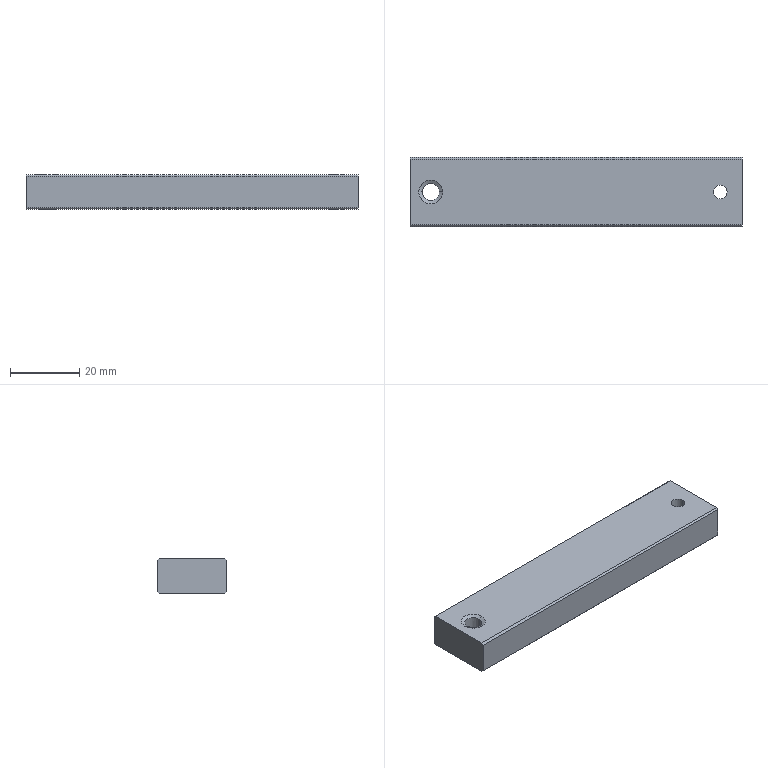Part | NX | 1 solid | 30 faces | box 96 x 20 x 10 mm | volume 18717 mm3 | cylinder 12 | plane 10 | cone 8 | commonest cylinder face diameters 3.3 x8 4 x2 5 x2
STEP:
#1=CARTESIAN_POINT('',(-48.,-9.5,5.));
#2=VERTEX_POINT('',#1);
#3=CARTESIAN_POINT('',(48.,-9.5,5.));
#4=VERTEX_POINT('',#3);
#5=CARTESIAN_POINT('',(0.,-9.5,5.));
#6=DIRECTION('',(1.,0.,0.));
#7=VECTOR('',#6,1000.);
#8=LINE('',#5,#7);
#9=EDGE_CURVE('',#2,#4,#8,.T.);
#10=ORIENTED_EDGE('',*,*,#9,.T.);
#11=CARTESIAN_POINT('',(48.,9.5,5.));
#12=VERTEX_POINT('',#11);
#13=CARTESIAN_POINT('',(48.,0.,5.));
#14=DIRECTION('',(0.,-1.,0.));
#15=VECTOR('',#14,1000.);
#16=LINE('',#13,#15);
#17=EDGE_CURVE('',#12,#4,#16,.T.);
#18=ORIENTED_EDGE('',*,*,#17,.F.);
#19=CARTESIAN_POINT('',(-48.,9.5,5.));
#20=VERTEX_POINT('',#19);
#21=CARTESIAN_POINT('',(0.,9.5,5.));
#22=DIRECTION('',(-1.,0.,0.));
#23=VECTOR('',#22,1000.);
#24=LINE('',#21,#23);
#25=EDGE_CURVE('',#12,#20,#24,.T.);
#26=ORIENTED_EDGE('',*,*,#25,.T.);
#27=CARTESIAN_POINT('',(-48.,0.,5.));
#28=DIRECTION('',(0.,1.,0.));
#29=VECTOR('',#28,1000.);
#30=LINE('',#27,#29);
#31=EDGE_CURVE('',#2,#20,#30,.T.);
#32=ORIENTED_EDGE('',*,*,#31,.F.);
#33=EDGE_LOOP('',(#10,#18,#26,#32));
#34=FACE_BOUND('',#33,.T.);
#35=CARTESIAN_POINT('',(43.7,0.,5.));
#36=VERTEX_POINT('',#35);
#37=CARTESIAN_POINT('',(39.7,0.,5.));
#38=VERTEX_POINT('',#37);
#39=CARTESIAN_POINT('',(41.7,0.,5.));
#40=DIRECTION('',(0.,0.,-1.));
#41=DIRECTION('',(-1.,0.,0.));
#42=AXIS2_PLACEMENT_3D('',#39,#40,#41);
#43=CIRCLE('',#42,2.);
#44=EDGE_CURVE('',#36,#38,#43,.T.);
#45=ORIENTED_EDGE('',*,*,#44,.T.);
#46=CARTESIAN_POINT('',(41.7,0.,5.));
#47=DIRECTION('',(0.,0.,-1.));
#48=DIRECTION('',(-1.,0.,0.));
#49=AXIS2_PLACEMENT_3D('',#46,#47,#48);
#50=CIRCLE('',#49,2.);
#51=EDGE_CURVE('',#38,#36,#50,.T.);
#52=ORIENTED_EDGE('',*,*,#51,.T.);
#53=EDGE_LOOP('',(#45,#52));
#54=FACE_BOUND('',#53,.T.);
#55=CARTESIAN_POINT('',(-45.45,0.,5.));
#56=VERTEX_POINT('',#55);
#57=CARTESIAN_POINT('',(-38.55,0.,5.));
#58=VERTEX_POINT('',#57);
#59=CARTESIAN_POINT('',(-42.,0.,5.));
#60=DIRECTION('',(0.,0.,1.));
#61=DIRECTION('',(1.,0.,0.));
#62=AXIS2_PLACEMENT_3D('',#59,#60,#61);
#63=CIRCLE('',#62,3.45);
#64=EDGE_CURVE('',#56,#58,#63,.T.);
#65=ORIENTED_EDGE('',*,*,#64,.F.);
#66=CARTESIAN_POINT('',(-42.,0.,5.));
#67=DIRECTION('',(0.,0.,1.));
#68=DIRECTION('',(1.,0.,0.));
#69=AXIS2_PLACEMENT_3D('',#66,#67,#68);
#70=CIRCLE('',#69,3.45);
#71=EDGE_CURVE('',#58,#56,#70,.T.);
#72=ORIENTED_EDGE('',*,*,#71,.F.);
#73=EDGE_LOOP('',(#65,#72));
#74=FACE_BOUND('',#73,.T.);
#75=CARTESIAN_POINT('',(0.,0.,5.));
#76=DIRECTION('',(0.,0.,1.));
#77=DIRECTION('',(1.,0.,0.));
#78=AXIS2_PLACEMENT_3D('',#75,#76,#77);
#79=PLANE('',#78);
#80=ADVANCED_FACE('',(#34,#54,#74),#79,.T.);
#81=ORIENTED_EDGE('',*,*,#31,.T.);
#82=CARTESIAN_POINT('',(-48.,10.,4.5));
#83=VERTEX_POINT('',#82);
#84=CARTESIAN_POINT('',(-48.,14.5,0.));
#85=DIRECTION('',(0.,0.7071,-0.7071));
#86=VECTOR('',#85,1000.);
#87=LINE('',#84,#86);
#88=EDGE_CURVE('',#20,#83,#87,.T.);
#89=ORIENTED_EDGE('',*,*,#88,.T.);
#90=CARTESIAN_POINT('',(-48.,10.,-4.5));
#91=VERTEX_POINT('',#90);
#92=CARTESIAN_POINT('',(-48.,10.,0.));
#93=DIRECTION('',(0.,0.,-1.));
#94=VECTOR('',#93,1000.);
#95=LINE('',#92,#94);
#96=EDGE_CURVE('',#83,#91,#95,.T.);
#97=ORIENTED_EDGE('',*,*,#96,.T.);
#98=CARTESIAN_POINT('',(-48.,9.5,-5.));
#99=VERTEX_POINT('',#98);
#100=CARTESIAN_POINT('',(-48.,14.5,0.));
#101=DIRECTION('',(0.,-0.7071,-0.7071));
#102=VECTOR('',#101,1000.);
#103=LINE('',#100,#102);
#104=EDGE_CURVE('',#91,#99,#103,.T.);
#105=ORIENTED_EDGE('',*,*,#104,.T.);
#106=CARTESIAN_POINT('',(-48.,-9.5,-5.));
#107=VERTEX_POINT('',#106);
#108=CARTESIAN_POINT('',(-48.,0.,-5.));
#109=DIRECTION('',(0.,1.,0.));
#110=VECTOR('',#109,1000.);
#111=LINE('',#108,#110);
#112=EDGE_CURVE('',#107,#99,#111,.T.);
#113=ORIENTED_EDGE('',*,*,#112,.F.);
#114=CARTESIAN_POINT('',(-48.,-10.,-4.5));
#115=VERTEX_POINT('',#114);
#116=CARTESIAN_POINT('',(-48.,-14.5,0.));
#117=DIRECTION('',(0.,-0.7071,0.7071));
#118=VECTOR('',#117,1000.);
#119=LINE('',#116,#118);
#120=EDGE_CURVE('',#107,#115,#119,.T.);
#121=ORIENTED_EDGE('',*,*,#120,.T.);
#122=CARTESIAN_POINT('',(-48.,-10.,4.5));
#123=VERTEX_POINT('',#122);
#124=CARTESIAN_POINT('',(-48.,-10.,0.));
#125=DIRECTION('',(0.,0.,1.));
#126=VECTOR('',#125,1000.);
#127=LINE('',#124,#126);
#128=EDGE_CURVE('',#115,#123,#127,.T.);
#129=ORIENTED_EDGE('',*,*,#128,.T.);
#130=CARTESIAN_POINT('',(-48.,-14.5,0.));
#131=DIRECTION('',(0.,0.7071,0.7071));
#132=VECTOR('',#131,1000.);
#133=LINE('',#130,#132);
#134=EDGE_CURVE('',#123,#2,#133,.T.);
#135=ORIENTED_EDGE('',*,*,#134,.T.);
#136=EDGE_LOOP('',(#81,#89,#97,#105,#113,#121,#129,#135));
#137=FACE_BOUND('',#136,.T.);
#138=CARTESIAN_POINT('',(-48.,10.,-5.));
#139=DIRECTION('',(-1.,0.,0.));
#140=DIRECTION('',(0.,0.,1.));
#141=AXIS2_PLACEMENT_3D('',#138,#139,#140);
#142=PLANE('',#141);
#143=ADVANCED_FACE('',(#137),#142,.T.);
#144=CARTESIAN_POINT('',(48.,10.,4.5));
#145=VERTEX_POINT('',#144);
#146=CARTESIAN_POINT('',(0.,10.,4.5));
#147=DIRECTION('',(1.,0.,0.));
#148=VECTOR('',#147,1000.);
#149=LINE('',#146,#148);
#150=EDGE_CURVE('',#83,#145,#149,.T.);
#151=ORIENTED_EDGE('',*,*,#150,.T.);
#152=CARTESIAN_POINT('',(48.,10.,-4.5));
#153=VERTEX_POINT('',#152);
#154=CARTESIAN_POINT('',(48.,10.,0.));
#155=DIRECTION('',(0.,0.,1.));
#156=VECTOR('',#155,1000.);
#157=LINE('',#154,#156);
#158=EDGE_CURVE('',#153,#145,#157,.T.);
#159=ORIENTED_EDGE('',*,*,#158,.F.);
#160=CARTESIAN_POINT('',(0.,10.,-4.5));
#161=DIRECTION('',(-1.,0.,0.));
#162=VECTOR('',#161,1000.);
#163=LINE('',#160,#162);
#164=EDGE_CURVE('',#153,#91,#163,.T.);
#165=ORIENTED_EDGE('',*,*,#164,.T.);
#166=ORIENTED_EDGE('',*,*,#96,.F.);
#167=EDGE_LOOP('',(#151,#159,#165,#166));
#168=FACE_BOUND('',#167,.T.);
#169=CARTESIAN_POINT('',(-39.685,10.,0.));
#170=VERTEX_POINT('',#169);
#171=CARTESIAN_POINT('',(-44.315,10.,0.));
#172=VERTEX_POINT('',#171);
#173=CARTESIAN_POINT('',(-42.,10.,0.));
#174=DIRECTION('',(0.,1.,0.));
#175=DIRECTION('',(1.,0.,0.));
#176=AXIS2_PLACEMENT_3D('',#173,#174,#175);
#177=CIRCLE('',#176,2.315);
#178=EDGE_CURVE('',#170,#172,#177,.T.);
#179=ORIENTED_EDGE('',*,*,#178,.F.);
#180=CARTESIAN_POINT('',(-42.,10.,0.));
#181=DIRECTION('',(0.,1.,0.));
#182=DIRECTION('',(1.,0.,0.));
#183=AXIS2_PLACEMENT_3D('',#180,#181,#182);
#184=CIRCLE('',#183,2.315);
#185=EDGE_CURVE('',#172,#170,#184,.T.);
#186=ORIENTED_EDGE('',*,*,#185,.F.);
#187=EDGE_LOOP('',(#179,#186));
#188=FACE_BOUND('',#187,.T.);
#189=CARTESIAN_POINT('',(48.,10.,-5.));
#190=DIRECTION('',(0.,1.,0.));
#191=DIRECTION('',(1.,0.,0.));
#192=AXIS2_PLACEMENT_3D('',#189,#190,#191);
#193=PLANE('',#192);
#194=ADVANCED_FACE('',(#168,#188),#193,.T.);
#195=CARTESIAN_POINT('',(48.,-10.,4.5));
#196=VERTEX_POINT('',#195);
#197=CARTESIAN_POINT('',(48.,-10.,-4.5));
#198=VERTEX_POINT('',#197);
#199=CARTESIAN_POINT('',(48.,-10.,0.));
#200=DIRECTION('',(0.,0.,-1.));
#201=VECTOR('',#200,1000.);
#202=LINE('',#199,#201);
#203=EDGE_CURVE('',#196,#198,#202,.T.);
#204=ORIENTED_EDGE('',*,*,#203,.T.);
#205=CARTESIAN_POINT('',(48.,-9.5,-5.));
#206=VERTEX_POINT('',#205);
#207=CARTESIAN_POINT('',(48.,-14.5,0.));
#208=DIRECTION('',(0.,0.7071,-0.7071));
#209=VECTOR('',#208,1000.);
#210=LINE('',#207,#209);
#211=EDGE_CURVE('',#198,#206,#210,.T.);
#212=ORIENTED_EDGE('',*,*,#211,.T.);
#213=CARTESIAN_POINT('',(48.,9.5,-5.));
#214=VERTEX_POINT('',#213);
#215=CARTESIAN_POINT('',(48.,0.,-5.));
#216=DIRECTION('',(0.,-1.,0.));
#217=VECTOR('',#216,1000.);
#218=LINE('',#215,#217);
#219=EDGE_CURVE('',#214,#206,#218,.T.);
#220=ORIENTED_EDGE('',*,*,#219,.F.);
#221=CARTESIAN_POINT('',(48.,14.5,0.));
#222=DIRECTION('',(0.,0.7071,0.7071));
#223=VECTOR('',#222,1000.);
#224=LINE('',#221,#223);
#225=EDGE_CURVE('',#214,#153,#224,.T.);
#226=ORIENTED_EDGE('',*,*,#225,.T.);
#227=ORIENTED_EDGE('',*,*,#158,.T.);
#228=CARTESIAN_POINT('',(48.,14.5,0.));
#229=DIRECTION('',(0.,-0.7071,0.7071));
#230=VECTOR('',#229,1000.);
#231=LINE('',#228,#230);
#232=EDGE_CURVE('',#145,#12,#231,.T.);
#233=ORIENTED_EDGE('',*,*,#232,.T.);
#234=ORIENTED_EDGE('',*,*,#17,.T.);
#235=CARTESIAN_POINT('',(48.,-14.5,0.));
#236=DIRECTION('',(0.,-0.7071,-0.7071));
#237=VECTOR('',#236,1000.);
#238=LINE('',#235,#237);
#239=EDGE_CURVE('',#4,#196,#238,.T.);
#240=ORIENTED_EDGE('',*,*,#239,.T.);
#241=EDGE_LOOP('',(#204,#212,#220,#226,#227,#233,#234,#240));
#242=FACE_BOUND('',#241,.T.);
#243=CARTESIAN_POINT('',(48.,2.315,0.));
#244=VERTEX_POINT('',#243);
#245=CARTESIAN_POINT('',(48.,-2.315,0.));
#246=VERTEX_POINT('',#245);
#247=CARTESIAN_POINT('',(48.,0.,0.));
#248=DIRECTION('',(1.,0.,0.));
#249=DIRECTION('',(0.,-1.,0.));
#250=AXIS2_PLACEMENT_3D('',#247,#248,#249);
#251=CIRCLE('',#250,2.315);
#252=EDGE_CURVE('',#244,#246,#251,.T.);
#253=ORIENTED_EDGE('',*,*,#252,.F.);
#254=CARTESIAN_POINT('',(48.,0.,0.));
#255=DIRECTION('',(1.,0.,0.));
#256=DIRECTION('',(0.,-1.,0.));
#257=AXIS2_PLACEMENT_3D('',#254,#255,#256);
#258=CIRCLE('',#257,2.315);
#259=EDGE_CURVE('',#246,#244,#258,.T.);
#260=ORIENTED_EDGE('',*,*,#259,.F.);
#261=EDGE_LOOP('',(#253,#260));
#262=FACE_BOUND('',#261,.T.);
#263=CARTESIAN_POINT('',(48.,-10.,-5.));
#264=DIRECTION('',(1.,0.,0.));
#265=DIRECTION('',(0.,1.,0.));
#266=AXIS2_PLACEMENT_3D('',#263,#264,#265);
#267=PLANE('',#266);
#268=ADVANCED_FACE('',(#242,#262),#267,.T.);
#269=CARTESIAN_POINT('',(0.,-10.,4.5));
#270=DIRECTION('',(-1.,0.,0.));
#271=VECTOR('',#270,1000.);
#272=LINE('',#269,#271);
#273=EDGE_CURVE('',#196,#123,#272,.T.);
#274=ORIENTED_EDGE('',*,*,#273,.T.);
#275=ORIENTED_EDGE('',*,*,#128,.F.);
#276=CARTESIAN_POINT('',(0.,-10.,-4.5));
#277=DIRECTION('',(1.,0.,0.));
#278=VECTOR('',#277,1000.);
#279=LINE('',#276,#278);
#280=EDGE_CURVE('',#115,#198,#279,.T.);
#281=ORIENTED_EDGE('',*,*,#280,.T.);
#282=ORIENTED_EDGE('',*,*,#203,.F.);
#283=EDGE_LOOP('',(#274,#275,#281,#282));
#284=FACE_BOUND('',#283,.T.);
#285=CARTESIAN_POINT('',(-48.,-10.,-5.));
#286=DIRECTION('',(0.,-1.,0.));
#287=DIRECTION('',(0.,0.,-1.));
#288=AXIS2_PLACEMENT_3D('',#285,#286,#287);
#289=PLANE('',#288);
#290=ADVANCED_FACE('',(#284),#289,.T.);
#291=CARTESIAN_POINT('',(0.,9.5,-5.));
#292=DIRECTION('',(-1.,0.,0.));
#293=VECTOR('',#292,1000.);
#294=LINE('',#291,#293);
#295=EDGE_CURVE('',#214,#99,#294,.T.);
#296=ORIENTED_EDGE('',*,*,#295,.T.);
#297=ORIENTED_EDGE('',*,*,#104,.F.);
#298=ORIENTED_EDGE('',*,*,#164,.F.);
#299=ORIENTED_EDGE('',*,*,#225,.F.);
#300=EDGE_LOOP('',(#296,#297,#298,#299));
#301=FACE_BOUND('',#300,.T.);
#302=CARTESIAN_POINT('',(0.,9.75,-4.75));
#303=DIRECTION('',(0.,-0.7071,0.7071));
#304=DIRECTION('',(-1.,0.,0.));
#305=AXIS2_PLACEMENT_3D('',#302,#303,#304);
#306=PLANE('',#305);
#307=ADVANCED_FACE('',(#301),#306,.F.);
#308=CARTESIAN_POINT('',(0.,-9.5,-5.));
#309=DIRECTION('',(1.,0.,0.));
#310=VECTOR('',#309,1000.);
#311=LINE('',#308,#310);
#312=EDGE_CURVE('',#107,#206,#311,.T.);
#313=ORIENTED_EDGE('',*,*,#312,.F.);
#314=ORIENTED_EDGE('',*,*,#112,.T.);
#315=ORIENTED_EDGE('',*,*,#295,.F.);
#316=ORIENTED_EDGE('',*,*,#219,.T.);
#317=EDGE_LOOP('',(#313,#314,#315,#316));
#318=FACE_BOUND('',#317,.T.);
#319=CARTESIAN_POINT('',(43.7,0.,-5.));
#320=VERTEX_POINT('',#319);
#321=CARTESIAN_POINT('',(39.7,0.,-5.));
#322=VERTEX_POINT('',#321);
#323=CARTESIAN_POINT('',(41.7,0.,-5.));
#324=DIRECTION('',(0.,0.,-1.));
#325=DIRECTION('',(-1.,0.,0.));
#326=AXIS2_PLACEMENT_3D('',#323,#324,#325);
#327=CIRCLE('',#326,2.);
#328=EDGE_CURVE('',#320,#322,#327,.T.);
#329=ORIENTED_EDGE('',*,*,#328,.F.);
#330=CARTESIAN_POINT('',(41.7,0.,-5.));
#331=DIRECTION('',(0.,0.,-1.));
#332=DIRECTION('',(-1.,0.,0.));
#333=AXIS2_PLACEMENT_3D('',#330,#331,#332);
#334=CIRCLE('',#333,2.);
#335=EDGE_CURVE('',#322,#320,#334,.T.);
#336=ORIENTED_EDGE('',*,*,#335,.F.);
#337=EDGE_LOOP('',(#329,#336));
#338=FACE_BOUND('',#337,.T.);
#339=CARTESIAN_POINT('',(-39.5,0.,-5.));
#340=VERTEX_POINT('',#339);
#341=CARTESIAN_POINT('',(-44.5,0.,-5.));
#342=VERTEX_POINT('',#341);
#343=CARTESIAN_POINT('',(-42.,0.,-5.));
#344=DIRECTION('',(0.,0.,1.));
#345=DIRECTION('',(1.,0.,0.));
#346=AXIS2_PLACEMENT_3D('',#343,#344,#345);
#347=CIRCLE('',#346,2.5);
#348=EDGE_CURVE('',#340,#342,#347,.T.);
#349=ORIENTED_EDGE('',*,*,#348,.T.);
#350=CARTESIAN_POINT('',(-42.,0.,-5.));
#351=DIRECTION('',(0.,0.,1.));
#352=DIRECTION('',(1.,0.,0.));
#353=AXIS2_PLACEMENT_3D('',#350,#351,#352);
#354=CIRCLE('',#353,2.5);
#355=EDGE_CURVE('',#342,#340,#354,.T.);
#356=ORIENTED_EDGE('',*,*,#355,.T.);
#357=EDGE_LOOP('',(#349,#356));
#358=FACE_BOUND('',#357,.T.);
#359=CARTESIAN_POINT('',(0.,0.,-5.));
#360=DIRECTION('',(0.,0.,1.));
#361=DIRECTION('',(1.,0.,0.));
#362=AXIS2_PLACEMENT_3D('',#359,#360,#361);
#363=PLANE('',#362);
#364=ADVANCED_FACE('',(#318,#338,#358),#363,.F.);
#365=ORIENTED_EDGE('',*,*,#312,.T.);
#366=ORIENTED_EDGE('',*,*,#211,.F.);
#367=ORIENTED_EDGE('',*,*,#280,.F.);
#368=ORIENTED_EDGE('',*,*,#120,.F.);
#369=EDGE_LOOP('',(#365,#366,#367,#368));
#370=FACE_BOUND('',#369,.T.);
#371=CARTESIAN_POINT('',(0.,-9.75,-4.75));
#372=DIRECTION('',(0.,0.7071,0.7071));
#373=DIRECTION('',(1.,0.,0.));
#374=AXIS2_PLACEMENT_3D('',#371,#372,#373);
#375=PLANE('',#374);
#376=ADVANCED_FACE('',(#370),#375,.F.);
#377=CARTESIAN_POINT('',(47.616,1.65,0.));
#378=VERTEX_POINT('',#377);
#379=CARTESIAN_POINT('',(47.616,-1.65,0.));
#380=VERTEX_POINT('',#379);
#381=CARTESIAN_POINT('',(47.616,0.,0.));
#382=DIRECTION('',(1.,0.,0.));
#383=DIRECTION('',(0.,-1.,0.));
#384=AXIS2_PLACEMENT_3D('',#381,#382,#383);
#385=CIRCLE('',#384,1.65);
#386=EDGE_CURVE('',#378,#380,#385,.T.);
#387=ORIENTED_EDGE('',*,*,#386,.F.);
#388=CARTESIAN_POINT('',(47.616,1.65,0.));
#389=DIRECTION('',(0.5,0.866,0.));
#390=VECTOR('',#389,1000.);
#391=LINE('',#388,#390);
#392=EDGE_CURVE('',#244,#378,#391,.F.);
#393=ORIENTED_EDGE('',*,*,#392,.F.);
#394=ORIENTED_EDGE('',*,*,#252,.T.);
#395=CARTESIAN_POINT('',(47.616,-1.65,0.));
#396=DIRECTION('',(0.5,-0.866,0.));
#397=VECTOR('',#396,1000.);
#398=LINE('',#395,#397);
#399=EDGE_CURVE('',#246,#380,#398,.F.);
#400=ORIENTED_EDGE('',*,*,#399,.T.);
#401=EDGE_LOOP('',(#387,#393,#394,#400));
#402=FACE_BOUND('',#401,.T.);
#403=CARTESIAN_POINT('',(47.616,0.,0.));
#404=DIRECTION('',(1.,0.,0.));
#405=DIRECTION('',(0.,-1.,0.));
#406=AXIS2_PLACEMENT_3D('',#403,#404,#405);
#407=CONICAL_SURFACE('',#406,1.65,1.047);
#408=ADVANCED_FACE('',(#402),#407,.F.);
#409=ORIENTED_EDGE('',*,*,#9,.F.);
#410=ORIENTED_EDGE('',*,*,#134,.F.);
#411=ORIENTED_EDGE('',*,*,#273,.F.);
#412=ORIENTED_EDGE('',*,*,#239,.F.);
#413=EDGE_LOOP('',(#409,#410,#411,#412));
#414=FACE_BOUND('',#413,.T.);
#415=CARTESIAN_POINT('',(0.,-9.75,4.75));
#416=DIRECTION('',(0.,0.7071,-0.7071));
#417=DIRECTION('',(-1.,0.,0.));
#418=AXIS2_PLACEMENT_3D('',#415,#416,#417);
#419=PLANE('',#418);
#420=ADVANCED_FACE('',(#414),#419,.F.);
#421=ORIENTED_EDGE('',*,*,#25,.F.);
#422=ORIENTED_EDGE('',*,*,#232,.F.);
#423=ORIENTED_EDGE('',*,*,#150,.F.);
#424=ORIENTED_EDGE('',*,*,#88,.F.);
#425=EDGE_LOOP('',(#421,#422,#423,#424));
#426=FACE_BOUND('',#425,.T.);
#427=CARTESIAN_POINT('',(0.,9.75,4.75));
#428=DIRECTION('',(0.,-0.7071,-0.7071));
#429=DIRECTION('',(0.,-0.7071,0.7071));
#430=AXIS2_PLACEMENT_3D('',#427,#428,#429);
#431=PLANE('',#430);
#432=ADVANCED_FACE('',(#426),#431,.F.);
#433=ORIENTED_EDGE('',*,*,#44,.F.);
#434=CARTESIAN_POINT('',(43.7,0.,1.65));
#435=VERTEX_POINT('',#434);
#436=CARTESIAN_POINT('',(43.7,0.,5.));
#437=DIRECTION('',(0.,0.,-1.));
#438=VECTOR('',#437,1000.);
#439=LINE('',#436,#438);
#440=EDGE_CURVE('',#36,#435,#439,.T.);
#441=ORIENTED_EDGE('',*,*,#440,.T.);
#442=CARTESIAN_POINT('',(42.83,-1.65,0.));
#443=VERTEX_POINT('',#442);
#444=CARTESIAN_POINT('',(43.7,0.,1.65));
#445=CARTESIAN_POINT('',(43.7,-0.4508,1.65));
#446=CARTESIAN_POINT('',(43.439,-1.102,1.339));
#447=CARTESIAN_POINT('',(42.983,-1.549,0.6815));
#448=CARTESIAN_POINT('',(42.83,-1.65,0.2103));
#449=CARTESIAN_POINT('',(42.83,-1.65,0.));
#450=B_SPLINE_CURVE_WITH_KNOTS('',3,(#444,#445,#446,#447,#448,#449),.UNSPECIFIED.,.F.,.F.,(4,1,1,4),(0.,0.5,0.75,1.),.UNSPECIFIED.);
#451=EDGE_CURVE('',#435,#443,#450,.T.);
#452=ORIENTED_EDGE('',*,*,#451,.T.);
#453=CARTESIAN_POINT('',(43.7,0.,-1.65));
#454=VERTEX_POINT('',#453);
#455=CARTESIAN_POINT('',(42.83,-1.65,0.));
#456=CARTESIAN_POINT('',(42.83,-1.65,-0.2102));
#457=CARTESIAN_POINT('',(42.983,-1.549,-0.6815));
#458=CARTESIAN_POINT('',(43.439,-1.102,-1.339));
#459=CARTESIAN_POINT('',(43.7,-0.451,-1.65));
#460=CARTESIAN_POINT('',(43.7,0.,-1.65));
#461=B_SPLINE_CURVE_WITH_KNOTS('',3,(#455,#456,#457,#458,#459,#460),.UNSPECIFIED.,.F.,.F.,(4,1,1,4),(0.,0.25,0.5,1.),.UNSPECIFIED.);
#462=EDGE_CURVE('',#443,#454,#461,.T.);
#463=ORIENTED_EDGE('',*,*,#462,.T.);
#464=CARTESIAN_POINT('',(43.7,0.,5.));
#465=DIRECTION('',(0.,0.,-1.));
#466=VECTOR('',#465,1000.);
#467=LINE('',#464,#466);
#468=EDGE_CURVE('',#454,#320,#467,.T.);
#469=ORIENTED_EDGE('',*,*,#468,.T.);
#470=ORIENTED_EDGE('',*,*,#328,.T.);
#471=CARTESIAN_POINT('',(39.7,0.,5.));
#472=DIRECTION('',(0.,0.,-1.));
#473=VECTOR('',#472,1000.);
#474=LINE('',#471,#473);
#475=EDGE_CURVE('',#38,#322,#474,.T.);
#476=ORIENTED_EDGE('',*,*,#475,.F.);
#477=EDGE_LOOP('',(#433,#441,#452,#463,#469,#470,#476));
#478=FACE_BOUND('',#477,.T.);
#479=CARTESIAN_POINT('',(41.7,0.,5.));
#480=DIRECTION('',(0.,0.,-1.));
#481=DIRECTION('',(-1.,0.,0.));
#482=AXIS2_PLACEMENT_3D('',#479,#480,#481);
#483=CYLINDRICAL_SURFACE('',#482,2.);
#484=ADVANCED_FACE('',(#478),#483,.F.);
#485=ORIENTED_EDGE('',*,*,#386,.T.);
#486=CARTESIAN_POINT('',(48.,-1.65,0.));
#487=DIRECTION('',(1.,0.,0.));
#488=VECTOR('',#487,1000.);
#489=LINE('',#486,#488);
#490=EDGE_CURVE('',#380,#443,#489,.F.);
#491=ORIENTED_EDGE('',*,*,#490,.T.);
#492=ORIENTED_EDGE('',*,*,#451,.F.);
#493=CARTESIAN_POINT('',(42.83,1.65,0.));
#494=VERTEX_POINT('',#493);
#495=CARTESIAN_POINT('',(43.7,0.,1.65));
#496=CARTESIAN_POINT('',(43.7,0.2195,1.65));
#497=CARTESIAN_POINT('',(43.625,0.5988,1.558));
#498=CARTESIAN_POINT('',(43.489,0.9084,1.39));
#499=CARTESIAN_POINT('',(43.256,1.288,1.076));
#500=CARTESIAN_POINT('',(42.987,1.542,0.6894));
#501=CARTESIAN_POINT('',(42.83,1.65,0.2066));
#502=CARTESIAN_POINT('',(42.83,1.65,0.));
#503=B_SPLINE_CURVE_WITH_KNOTS('',3,(#495,#496,#497,#498,#499,#500,#501,#502),.UNSPECIFIED.,.F.,.F.,(4,1,1,1,1,4),(0.,0.25,0.375,0.5,0.75,1.),.UNSPECIFIED.);
#504=EDGE_CURVE('',#494,#435,#503,.F.);
#505=ORIENTED_EDGE('',*,*,#504,.F.);
#506=CARTESIAN_POINT('',(48.,1.65,0.));
#507=DIRECTION('',(1.,0.,0.));
#508=VECTOR('',#507,1000.);
#509=LINE('',#506,#508);
#510=EDGE_CURVE('',#378,#494,#509,.F.);
#511=ORIENTED_EDGE('',*,*,#510,.F.);
#512=EDGE_LOOP('',(#485,#491,#492,#505,#511));
#513=FACE_BOUND('',#512,.T.);
#514=CARTESIAN_POINT('',(48.,0.,0.));
#515=DIRECTION('',(1.,0.,0.));
#516=DIRECTION('',(0.,-1.,0.));
#517=AXIS2_PLACEMENT_3D('',#514,#515,#516);
#518=CYLINDRICAL_SURFACE('',#517,1.65);
#519=ADVANCED_FACE('',(#513),#518,.F.);
#520=ORIENTED_EDGE('',*,*,#348,.F.);
#521=CARTESIAN_POINT('',(-39.5,0.,4.452));
#522=VERTEX_POINT('',#521);
#523=CARTESIAN_POINT('',(-39.5,0.,5.));
#524=DIRECTION('',(0.,0.,1.));
#525=VECTOR('',#524,1000.);
#526=LINE('',#523,#525);
#527=EDGE_CURVE('',#340,#522,#526,.T.);
#528=ORIENTED_EDGE('',*,*,#527,.T.);
#529=CARTESIAN_POINT('',(-44.5,0.,4.452));
#530=VERTEX_POINT('',#529);
#531=CARTESIAN_POINT('',(-42.,0.,4.452));
#532=DIRECTION('',(0.,0.,1.));
#533=DIRECTION('',(1.,0.,0.));
#534=AXIS2_PLACEMENT_3D('',#531,#532,#533);
#535=CIRCLE('',#534,2.5);
#536=EDGE_CURVE('',#522,#530,#535,.T.);
#537=ORIENTED_EDGE('',*,*,#536,.T.);
#538=CARTESIAN_POINT('',(-44.5,0.,5.));
#539=DIRECTION('',(0.,0.,1.));
#540=VECTOR('',#539,1000.);
#541=LINE('',#538,#540);
#542=EDGE_CURVE('',#342,#530,#541,.T.);
#543=ORIENTED_EDGE('',*,*,#542,.F.);
#544=EDGE_LOOP('',(#520,#528,#537,#543));
#545=FACE_BOUND('',#544,.T.);
#546=CARTESIAN_POINT('',(-40.35,1.878,0.));
#547=VERTEX_POINT('',#546);
#548=CARTESIAN_POINT('',(-43.5,2.,0.6874));
#549=VERTEX_POINT('',#548);
#550=CARTESIAN_POINT('',(-43.5,2.,0.6874));
#551=CARTESIAN_POINT('',(-43.345,2.116,1.026));
#552=CARTESIAN_POINT('',(-42.838,2.442,1.573));
#553=CARTESIAN_POINT('',(-41.184,2.613,1.808));
#554=CARTESIAN_POINT('',(-40.35,1.878,0.7403));
#555=CARTESIAN_POINT('',(-40.35,1.878,0.));
#556=B_SPLINE_CURVE_WITH_KNOTS('',3,(#550,#551,#552,#553,#554,#555),.UNSPECIFIED.,.F.,.F.,(4,1,1,4),(0.,0.25,0.5,1.),.UNSPECIFIED.);
#557=EDGE_CURVE('',#547,#549,#556,.F.);
#558=ORIENTED_EDGE('',*,*,#557,.F.);
#559=CARTESIAN_POINT('',(-43.5,2.,-0.6874));
#560=VERTEX_POINT('',#559);
#561=CARTESIAN_POINT('',(-40.35,1.878,0.));
#562=CARTESIAN_POINT('',(-40.35,1.878,-0.7402));
#563=CARTESIAN_POINT('',(-41.184,2.613,-1.808));
#564=CARTESIAN_POINT('',(-42.838,2.442,-1.573));
#565=CARTESIAN_POINT('',(-43.345,2.116,-1.026));
#566=CARTESIAN_POINT('',(-43.5,2.,-0.6874));
#567=B_SPLINE_CURVE_WITH_KNOTS('',3,(#561,#562,#563,#564,#565,#566),.UNSPECIFIED.,.F.,.F.,(4,1,1,4),(0.,0.5,0.75,1.),.UNSPECIFIED.);
#568=EDGE_CURVE('',#560,#547,#567,.F.);
#569=ORIENTED_EDGE('',*,*,#568,.F.);
#570=CARTESIAN_POINT('',(-43.65,1.878,0.));
#571=VERTEX_POINT('',#570);
#572=CARTESIAN_POINT('',(-43.65,1.878,0.));
#573=CARTESIAN_POINT('',(-43.65,1.878,-0.05991));
#574=CARTESIAN_POINT('',(-43.647,1.881,-0.1201));
#575=CARTESIAN_POINT('',(-43.64,1.887,-0.1798));
#576=CARTESIAN_POINT('',(-43.634,1.892,-0.2395));
#577=CARTESIAN_POINT('',(-43.624,1.901,-0.2987));
#578=CARTESIAN_POINT('',(-43.611,1.912,-0.3566));
#579=CARTESIAN_POINT('',(-43.598,1.923,-0.4145));
#580=CARTESIAN_POINT('',(-43.582,1.936,-0.4707));
#581=CARTESIAN_POINT('',(-43.564,1.95,-0.5259));
#582=CARTESIAN_POINT('',(-43.545,1.965,-0.5811));
#583=CARTESIAN_POINT('',(-43.524,1.982,-0.635));
#584=CARTESIAN_POINT('',(-43.5,2.,-0.6874));
#585=B_SPLINE_CURVE_WITH_KNOTS('',3,(#572,#573,#574,#575,#576,#577,#578,#579,#580,#581,#582,#583,#584),.UNSPECIFIED.,.F.,.F.,(4,3,3,3,4),(0.,0.1804,0.3614,0.5416,0.7223),.UNSPECIFIED.);
#586=EDGE_CURVE('',#571,#560,#585,.T.);
#587=ORIENTED_EDGE('',*,*,#586,.F.);
#588=CARTESIAN_POINT('',(-43.5,2.,0.6874));
#589=CARTESIAN_POINT('',(-43.524,1.982,0.635));
#590=CARTESIAN_POINT('',(-43.545,1.965,0.5811));
#591=CARTESIAN_POINT('',(-43.564,1.95,0.5259));
#592=CARTESIAN_POINT('',(-43.582,1.936,0.4707));
#593=CARTESIAN_POINT('',(-43.598,1.923,0.4145));
#594=CARTESIAN_POINT('',(-43.611,1.912,0.3566));
#595=CARTESIAN_POINT('',(-43.624,1.901,0.2987));
#596=CARTESIAN_POINT('',(-43.634,1.892,0.2395));
#597=CARTESIAN_POINT('',(-43.64,1.887,0.1798));
#598=CARTESIAN_POINT('',(-43.647,1.881,0.1201));
#599=CARTESIAN_POINT('',(-43.65,1.878,0.05991));
#600=CARTESIAN_POINT('',(-43.65,1.878,0.));
#601=B_SPLINE_CURVE_WITH_KNOTS('',3,(#588,#589,#590,#591,#592,#593,#594,#595,#596,#597,#598,#599,#600),.UNSPECIFIED.,.F.,.F.,(4,3,3,3,4),(0.,0.1807,0.3608,0.5418,0.7223),.UNSPECIFIED.);
#602=EDGE_CURVE('',#549,#571,#601,.T.);
#603=ORIENTED_EDGE('',*,*,#602,.F.);
#604=EDGE_LOOP('',(#558,#569,#587,#603));
#605=FACE_BOUND('',#604,.T.);
#606=CARTESIAN_POINT('',(-42.,0.,5.));
#607=DIRECTION('',(0.,0.,1.));
#608=DIRECTION('',(1.,0.,0.));
#609=AXIS2_PLACEMENT_3D('',#606,#607,#608);
#610=CYLINDRICAL_SURFACE('',#609,2.5);
#611=ADVANCED_FACE('',(#545,#605),#610,.F.);
#612=CARTESIAN_POINT('',(-43.65,-2.2,0.));
#613=VERTEX_POINT('',#612);
#614=CARTESIAN_POINT('',(-43.187,-2.2,1.146));
#615=VERTEX_POINT('',#614);
#616=CARTESIAN_POINT('',(-42.,-2.2,0.));
#617=DIRECTION('',(0.,1.,0.));
#618=DIRECTION('',(1.,0.,0.));
#619=AXIS2_PLACEMENT_3D('',#616,#617,#618);
#620=CIRCLE('',#619,1.65);
#621=EDGE_CURVE('',#613,#615,#620,.T.);
#622=ORIENTED_EDGE('',*,*,#621,.T.);
#623=CARTESIAN_POINT('',(-40.813,-2.2,1.146));
#624=VERTEX_POINT('',#623);
#625=CARTESIAN_POINT('',(-40.813,-2.2,1.145));
#626=CARTESIAN_POINT('',(-41.01,-2.306,1.103));
#627=CARTESIAN_POINT('',(-41.206,-2.4,1.109));
#628=CARTESIAN_POINT('',(-41.819,-2.503,1.147));
#629=CARTESIAN_POINT('',(-42.,-2.498,1.152));
#630=CARTESIAN_POINT('',(-42.181,-2.503,1.147));
#631=CARTESIAN_POINT('',(-42.794,-2.4,1.109));
#632=CARTESIAN_POINT('',(-42.992,-2.305,1.103));
#633=CARTESIAN_POINT('',(-43.187,-2.2,1.145));
#634=B_SPLINE_CURVE_WITH_KNOTS('',3,(#625,#626,#627,#628,#629,#630,#631,#632,#633),.UNSPECIFIED.,.F.,.F.,(4,1,1,1,1,1,4),(0.,0.25,0.375,0.5,0.625,0.75,1.),.UNSPECIFIED.);
#635=EDGE_CURVE('',#624,#615,#634,.T.);
#636=ORIENTED_EDGE('',*,*,#635,.F.);
#637=CARTESIAN_POINT('',(-40.35,-2.2,0.));
#638=VERTEX_POINT('',#637);
#639=CARTESIAN_POINT('',(-42.,-2.2,0.));
#640=DIRECTION('',(0.,1.,0.));
#641=DIRECTION('',(1.,0.,0.));
#642=AXIS2_PLACEMENT_3D('',#639,#640,#641);
#643=CIRCLE('',#642,1.65);
#644=EDGE_CURVE('',#624,#638,#643,.T.);
#645=ORIENTED_EDGE('',*,*,#644,.T.);
#646=CARTESIAN_POINT('',(-42.,-3.191,0.));
#647=VERTEX_POINT('',#646);
#648=CARTESIAN_POINT('',(-40.35,-2.2,0.));
#649=DIRECTION('',(0.8572,0.515,0.));
#650=VECTOR('',#649,1000.);
#651=LINE('',#648,#650);
#652=EDGE_CURVE('',#638,#647,#651,.F.);
#653=ORIENTED_EDGE('',*,*,#652,.T.);
#654=CARTESIAN_POINT('',(-43.65,-2.2,0.));
#655=DIRECTION('',(-0.8572,0.515,0.));
#656=VECTOR('',#655,1000.);
#657=LINE('',#654,#656);
#658=EDGE_CURVE('',#613,#647,#657,.F.);
#659=ORIENTED_EDGE('',*,*,#658,.F.);
#660=EDGE_LOOP('',(#622,#636,#645,#653,#659));
#661=FACE_BOUND('',#660,.T.);
#662=CARTESIAN_POINT('',(-42.,-2.2,0.));
#663=DIRECTION('',(0.,1.,0.));
#664=DIRECTION('',(1.,0.,0.));
#665=AXIS2_PLACEMENT_3D('',#662,#663,#664);
#666=CONICAL_SURFACE('',#665,1.65,1.03);
#667=ADVANCED_FACE('',(#661),#666,.F.);
#668=CARTESIAN_POINT('',(-40.35,9.616,0.));
#669=VERTEX_POINT('',#668);
#670=CARTESIAN_POINT('',(-43.65,9.616,0.));
#671=VERTEX_POINT('',#670);
#672=CARTESIAN_POINT('',(-42.,9.616,0.));
#673=DIRECTION('',(0.,1.,0.));
#674=DIRECTION('',(1.,0.,0.));
#675=AXIS2_PLACEMENT_3D('',#672,#673,#674);
#676=CIRCLE('',#675,1.65);
#677=EDGE_CURVE('',#669,#671,#676,.T.);
#678=ORIENTED_EDGE('',*,*,#677,.F.);
#679=CARTESIAN_POINT('',(-40.35,9.616,0.));
#680=DIRECTION('',(0.866,0.5,0.));
#681=VECTOR('',#680,1000.);
#682=LINE('',#679,#681);
#683=EDGE_CURVE('',#669,#170,#682,.T.);
#684=ORIENTED_EDGE('',*,*,#683,.T.);
#685=ORIENTED_EDGE('',*,*,#178,.T.);
#686=CARTESIAN_POINT('',(-43.65,9.616,0.));
#687=DIRECTION('',(-0.866,0.5,0.));
#688=VECTOR('',#687,1000.);
#689=LINE('',#686,#688);
#690=EDGE_CURVE('',#671,#172,#689,.T.);
#691=ORIENTED_EDGE('',*,*,#690,.F.);
#692=EDGE_LOOP('',(#678,#684,#685,#691));
#693=FACE_BOUND('',#692,.T.);
#694=CARTESIAN_POINT('',(-42.,9.616,0.));
#695=DIRECTION('',(0.,1.,0.));
#696=DIRECTION('',(1.,0.,0.));
#697=AXIS2_PLACEMENT_3D('',#694,#695,#696);
#698=CONICAL_SURFACE('',#697,1.65,1.047);
#699=ADVANCED_FACE('',(#693),#698,.F.);
#700=ORIENTED_EDGE('',*,*,#602,.T.);
#701=CARTESIAN_POINT('',(-43.65,10.,0.));
#702=DIRECTION('',(0.,1.,0.));
#703=VECTOR('',#702,1000.);
#704=LINE('',#701,#703);
#705=EDGE_CURVE('',#671,#571,#704,.F.);
#706=ORIENTED_EDGE('',*,*,#705,.F.);
#707=CARTESIAN_POINT('',(-42.,9.616,0.));
#708=DIRECTION('',(0.,1.,0.));
#709=DIRECTION('',(1.,0.,0.));
#710=AXIS2_PLACEMENT_3D('',#707,#708,#709);
#711=CIRCLE('',#710,1.65);
#712=EDGE_CURVE('',#671,#669,#711,.T.);
#713=ORIENTED_EDGE('',*,*,#712,.T.);
#714=CARTESIAN_POINT('',(-40.35,10.,0.));
#715=DIRECTION('',(0.,1.,0.));
#716=VECTOR('',#715,1000.);
#717=LINE('',#714,#716);
#718=EDGE_CURVE('',#669,#547,#717,.F.);
#719=ORIENTED_EDGE('',*,*,#718,.T.);
#720=ORIENTED_EDGE('',*,*,#557,.T.);
#721=EDGE_LOOP('',(#700,#706,#713,#719,#720));
#722=FACE_BOUND('',#721,.T.);
#723=CARTESIAN_POINT('',(-42.,10.,0.));
#724=DIRECTION('',(0.,1.,0.));
#725=DIRECTION('',(1.,0.,0.));
#726=AXIS2_PLACEMENT_3D('',#723,#724,#725);
#727=CYLINDRICAL_SURFACE('',#726,1.65);
#728=ADVANCED_FACE('',(#722),#727,.F.);
#729=CARTESIAN_POINT('',(-40.813,-2.2,-1.146));
#730=VERTEX_POINT('',#729);
#731=CARTESIAN_POINT('',(-42.,-2.2,0.));
#732=DIRECTION('',(0.,1.,0.));
#733=DIRECTION('',(1.,0.,0.));
#734=AXIS2_PLACEMENT_3D('',#731,#732,#733);
#735=CIRCLE('',#734,1.65);
#736=EDGE_CURVE('',#638,#730,#735,.T.);
#737=ORIENTED_EDGE('',*,*,#736,.F.);
#738=CARTESIAN_POINT('',(-40.35,-1.878,0.));
#739=VERTEX_POINT('',#738);
#740=CARTESIAN_POINT('',(-40.35,10.,0.));
#741=DIRECTION('',(0.,1.,0.));
#742=VECTOR('',#741,1000.);
#743=LINE('',#740,#742);
#744=EDGE_CURVE('',#638,#739,#743,.T.);
#745=ORIENTED_EDGE('',*,*,#744,.T.);
#746=CARTESIAN_POINT('',(-40.35,-1.878,0.));
#747=CARTESIAN_POINT('',(-40.35,-1.878,-0.09898));
#748=CARTESIAN_POINT('',(-40.363,-1.892,-0.2971));
#749=CARTESIAN_POINT('',(-40.459,-1.969,-0.6009));
#750=CARTESIAN_POINT('',(-40.527,-2.021,-0.75));
#751=CARTESIAN_POINT('',(-40.636,-2.095,-0.9316));
#752=CARTESIAN_POINT('',(-40.654,-2.108,-0.9563));
#753=CARTESIAN_POINT('',(-40.75,-2.166,-1.08));
#754=CARTESIAN_POINT('',(-40.813,-2.2,-1.146));
#755=B_SPLINE_CURVE_WITH_KNOTS('',3,(#746,#747,#748,#749,#750,#751,#752,#753,#754),.UNSPECIFIED.,.F.,.F.,(4,1,1,1,1,1,4),(0.,0.25,0.5,0.625,0.75,0.875,1.),.UNSPECIFIED.);
#756=EDGE_CURVE('',#730,#739,#755,.F.);
#757=ORIENTED_EDGE('',*,*,#756,.F.);
#758=EDGE_LOOP('',(#737,#745,#757));
#759=FACE_BOUND('',#758,.T.);
#760=CARTESIAN_POINT('',(-42.,10.,0.));
#761=DIRECTION('',(0.,1.,0.));
#762=DIRECTION('',(1.,0.,0.));
#763=AXIS2_PLACEMENT_3D('',#760,#761,#762);
#764=CYLINDRICAL_SURFACE('',#763,1.65);
#765=ADVANCED_FACE('',(#759),#764,.F.);
#766=CARTESIAN_POINT('',(-43.65,-1.878,0.));
#767=VERTEX_POINT('',#766);
#768=CARTESIAN_POINT('',(-43.187,-2.2,-1.146));
#769=VERTEX_POINT('',#768);
#770=CARTESIAN_POINT('',(-43.187,-2.2,-1.146));
#771=CARTESIAN_POINT('',(-43.25,-2.166,-1.08));
#772=CARTESIAN_POINT('',(-43.346,-2.108,-0.9563));
#773=CARTESIAN_POINT('',(-43.364,-2.095,-0.9316));
#774=CARTESIAN_POINT('',(-43.473,-2.021,-0.7503));
#775=CARTESIAN_POINT('',(-43.541,-1.969,-0.5991));
#776=CARTESIAN_POINT('',(-43.633,-1.893,-0.3117));
#777=CARTESIAN_POINT('',(-43.65,-1.878,-0.1049));
#778=CARTESIAN_POINT('',(-43.65,-1.878,0.));
#779=B_SPLINE_CURVE_WITH_KNOTS('',3,(#770,#771,#772,#773,#774,#775,#776,#777,#778),.UNSPECIFIED.,.F.,.F.,(4,1,1,1,1,1,4),(0.,0.125,0.25,0.375,0.5,0.75,1.),.UNSPECIFIED.);
#780=EDGE_CURVE('',#767,#769,#779,.F.);
#781=ORIENTED_EDGE('',*,*,#780,.F.);
#782=CARTESIAN_POINT('',(-43.65,10.,0.));
#783=DIRECTION('',(0.,1.,0.));
#784=VECTOR('',#783,1000.);
#785=LINE('',#782,#784);
#786=EDGE_CURVE('',#613,#767,#785,.T.);
#787=ORIENTED_EDGE('',*,*,#786,.F.);
#788=CARTESIAN_POINT('',(-42.,-2.2,0.));
#789=DIRECTION('',(0.,1.,0.));
#790=DIRECTION('',(1.,0.,0.));
#791=AXIS2_PLACEMENT_3D('',#788,#789,#790);
#792=CIRCLE('',#791,1.65);
#793=EDGE_CURVE('',#769,#613,#792,.T.);
#794=ORIENTED_EDGE('',*,*,#793,.F.);
#795=EDGE_LOOP('',(#781,#787,#794));
#796=FACE_BOUND('',#795,.T.);
#797=CARTESIAN_POINT('',(-42.,10.,0.));
#798=DIRECTION('',(0.,1.,0.));
#799=DIRECTION('',(1.,0.,0.));
#800=AXIS2_PLACEMENT_3D('',#797,#798,#799);
#801=CYLINDRICAL_SURFACE('',#800,1.65);
#802=ADVANCED_FACE('',(#796),#801,.F.);
#803=ORIENTED_EDGE('',*,*,#64,.T.);
#804=CARTESIAN_POINT('',(-39.5,0.,4.452));
#805=DIRECTION('',(0.866,0.,0.5));
#806=VECTOR('',#805,1000.);
#807=LINE('',#804,#806);
#808=EDGE_CURVE('',#522,#58,#807,.T.);
#809=ORIENTED_EDGE('',*,*,#808,.F.);
#810=CARTESIAN_POINT('',(-42.,0.,4.452));
#811=DIRECTION('',(0.,0.,1.));
#812=DIRECTION('',(1.,0.,0.));
#813=AXIS2_PLACEMENT_3D('',#810,#811,#812);
#814=CIRCLE('',#813,2.5);
#815=EDGE_CURVE('',#530,#522,#814,.T.);
#816=ORIENTED_EDGE('',*,*,#815,.F.);
#817=CARTESIAN_POINT('',(-44.5,0.,4.452));
#818=DIRECTION('',(-0.866,0.,0.5));
#819=VECTOR('',#818,1000.);
#820=LINE('',#817,#819);
#821=EDGE_CURVE('',#530,#56,#820,.T.);
#822=ORIENTED_EDGE('',*,*,#821,.T.);
#823=EDGE_LOOP('',(#803,#809,#816,#822));
#824=FACE_BOUND('',#823,.T.);
#825=CARTESIAN_POINT('',(-42.,0.,4.452));
#826=DIRECTION('',(0.,0.,1.));
#827=DIRECTION('',(1.,0.,0.));
#828=AXIS2_PLACEMENT_3D('',#825,#826,#827);
#829=CONICAL_SURFACE('',#828,2.5,1.047);
#830=ADVANCED_FACE('',(#824),#829,.F.);
#831=ORIENTED_EDGE('',*,*,#536,.F.);
#832=ORIENTED_EDGE('',*,*,#808,.T.);
#833=ORIENTED_EDGE('',*,*,#71,.T.);
#834=ORIENTED_EDGE('',*,*,#821,.F.);
#835=EDGE_LOOP('',(#831,#832,#833,#834));
#836=FACE_BOUND('',#835,.T.);
#837=CARTESIAN_POINT('',(-42.,0.,4.452));
#838=DIRECTION('',(0.,0.,1.));
#839=DIRECTION('',(1.,0.,0.));
#840=AXIS2_PLACEMENT_3D('',#837,#838,#839);
#841=CONICAL_SURFACE('',#840,2.5,1.047);
#842=ADVANCED_FACE('',(#836),#841,.F.);
#843=ORIENTED_EDGE('',*,*,#744,.F.);
#844=ORIENTED_EDGE('',*,*,#644,.F.);
#845=CARTESIAN_POINT('',(-40.813,-2.2,1.146));
#846=CARTESIAN_POINT('',(-40.75,-2.166,1.08));
#847=CARTESIAN_POINT('',(-40.654,-2.108,0.9563));
#848=CARTESIAN_POINT('',(-40.636,-2.095,0.9316));
#849=CARTESIAN_POINT('',(-40.527,-2.021,0.7503));
#850=CARTESIAN_POINT('',(-40.459,-1.969,0.5991));
#851=CARTESIAN_POINT('',(-40.367,-1.893,0.3117));
#852=CARTESIAN_POINT('',(-40.35,-1.878,0.1049));
#853=CARTESIAN_POINT('',(-40.35,-1.878,0.));
#854=B_SPLINE_CURVE_WITH_KNOTS('',3,(#845,#846,#847,#848,#849,#850,#851,#852,#853),.UNSPECIFIED.,.F.,.F.,(4,1,1,1,1,1,4),(0.,0.125,0.25,0.375,0.5,0.75,1.),.UNSPECIFIED.);
#855=EDGE_CURVE('',#739,#624,#854,.F.);
#856=ORIENTED_EDGE('',*,*,#855,.F.);
#857=EDGE_LOOP('',(#843,#844,#856));
#858=FACE_BOUND('',#857,.T.);
#859=CARTESIAN_POINT('',(-42.,10.,0.));
#860=DIRECTION('',(0.,1.,0.));
#861=DIRECTION('',(1.,0.,0.));
#862=AXIS2_PLACEMENT_3D('',#859,#860,#861);
#863=CYLINDRICAL_SURFACE('',#862,1.65);
#864=ADVANCED_FACE('',(#858),#863,.F.);
#865=ORIENTED_EDGE('',*,*,#683,.F.);
#866=ORIENTED_EDGE('',*,*,#712,.F.);
#867=ORIENTED_EDGE('',*,*,#690,.T.);
#868=ORIENTED_EDGE('',*,*,#185,.T.);
#869=EDGE_LOOP('',(#865,#866,#867,#868));
#870=FACE_BOUND('',#869,.T.);
#871=CARTESIAN_POINT('',(-42.,9.616,0.));
#872=DIRECTION('',(0.,1.,0.));
#873=DIRECTION('',(1.,0.,0.));
#874=AXIS2_PLACEMENT_3D('',#871,#872,#873);
#875=CONICAL_SURFACE('',#874,1.65,1.047);
#876=ADVANCED_FACE('',(#870),#875,.F.);
#877=ORIENTED_EDGE('',*,*,#468,.F.);
#878=CARTESIAN_POINT('',(43.7,0.,-1.65));
#879=CARTESIAN_POINT('',(43.7,0.4508,-1.65));
#880=CARTESIAN_POINT('',(43.439,1.102,-1.339));
#881=CARTESIAN_POINT('',(42.983,1.549,-0.6815));
#882=CARTESIAN_POINT('',(42.83,1.65,-0.2103));
#883=CARTESIAN_POINT('',(42.83,1.65,0.));
#884=B_SPLINE_CURVE_WITH_KNOTS('',3,(#878,#879,#880,#881,#882,#883),.UNSPECIFIED.,.F.,.F.,(4,1,1,4),(0.,0.5,0.75,1.),.UNSPECIFIED.);
#885=EDGE_CURVE('',#454,#494,#884,.T.);
#886=ORIENTED_EDGE('',*,*,#885,.T.);
#887=ORIENTED_EDGE('',*,*,#504,.T.);
#888=ORIENTED_EDGE('',*,*,#440,.F.);
#889=ORIENTED_EDGE('',*,*,#51,.F.);
#890=ORIENTED_EDGE('',*,*,#475,.T.);
#891=ORIENTED_EDGE('',*,*,#335,.T.);
#892=EDGE_LOOP('',(#877,#886,#887,#888,#889,#890,#891));
#893=FACE_BOUND('',#892,.T.);
#894=CARTESIAN_POINT('',(41.7,0.,5.));
#895=DIRECTION('',(0.,0.,-1.));
#896=DIRECTION('',(-1.,0.,0.));
#897=AXIS2_PLACEMENT_3D('',#894,#895,#896);
#898=CYLINDRICAL_SURFACE('',#897,2.);
#899=ADVANCED_FACE('',(#893),#898,.F.);
#900=ORIENTED_EDGE('',*,*,#786,.T.);
#901=CARTESIAN_POINT('',(-43.65,-1.878,0.));
#902=CARTESIAN_POINT('',(-43.65,-1.878,0.09898));
#903=CARTESIAN_POINT('',(-43.637,-1.892,0.2971));
#904=CARTESIAN_POINT('',(-43.541,-1.969,0.6009));
#905=CARTESIAN_POINT('',(-43.473,-2.021,0.75));
#906=CARTESIAN_POINT('',(-43.364,-2.095,0.9316));
#907=CARTESIAN_POINT('',(-43.346,-2.108,0.9563));
#908=CARTESIAN_POINT('',(-43.25,-2.166,1.08));
#909=CARTESIAN_POINT('',(-43.187,-2.2,1.146));
#910=B_SPLINE_CURVE_WITH_KNOTS('',3,(#901,#902,#903,#904,#905,#906,#907,#908,#909),.UNSPECIFIED.,.F.,.F.,(4,1,1,1,1,1,4),(0.,0.25,0.5,0.625,0.75,0.875,1.),.UNSPECIFIED.);
#911=EDGE_CURVE('',#615,#767,#910,.F.);
#912=ORIENTED_EDGE('',*,*,#911,.F.);
#913=ORIENTED_EDGE('',*,*,#621,.F.);
#914=EDGE_LOOP('',(#900,#912,#913));
#915=FACE_BOUND('',#914,.T.);
#916=CARTESIAN_POINT('',(-42.,10.,0.));
#917=DIRECTION('',(0.,1.,0.));
#918=DIRECTION('',(1.,0.,0.));
#919=AXIS2_PLACEMENT_3D('',#916,#917,#918);
#920=CYLINDRICAL_SURFACE('',#919,1.65);
#921=ADVANCED_FACE('',(#915),#920,.F.);
#922=ORIENTED_EDGE('',*,*,#677,.T.);
#923=ORIENTED_EDGE('',*,*,#705,.T.);
#924=ORIENTED_EDGE('',*,*,#586,.T.);
#925=ORIENTED_EDGE('',*,*,#568,.T.);
#926=ORIENTED_EDGE('',*,*,#718,.F.);
#927=EDGE_LOOP('',(#922,#923,#924,#925,#926));
#928=FACE_BOUND('',#927,.T.);
#929=CARTESIAN_POINT('',(-42.,10.,0.));
#930=DIRECTION('',(0.,1.,0.));
#931=DIRECTION('',(1.,0.,0.));
#932=AXIS2_PLACEMENT_3D('',#929,#930,#931);
#933=CYLINDRICAL_SURFACE('',#932,1.65);
#934=ADVANCED_FACE('',(#928),#933,.F.);
#935=ORIENTED_EDGE('',*,*,#399,.F.);
#936=ORIENTED_EDGE('',*,*,#259,.T.);
#937=ORIENTED_EDGE('',*,*,#392,.T.);
#938=CARTESIAN_POINT('',(47.616,0.,0.));
#939=DIRECTION('',(1.,0.,0.));
#940=DIRECTION('',(0.,-1.,0.));
#941=AXIS2_PLACEMENT_3D('',#938,#939,#940);
#942=CIRCLE('',#941,1.65);
#943=EDGE_CURVE('',#380,#378,#942,.T.);
#944=ORIENTED_EDGE('',*,*,#943,.F.);
#945=EDGE_LOOP('',(#935,#936,#937,#944));
#946=FACE_BOUND('',#945,.T.);
#947=CARTESIAN_POINT('',(47.616,0.,0.));
#948=DIRECTION('',(1.,0.,0.));
#949=DIRECTION('',(0.,-1.,0.));
#950=AXIS2_PLACEMENT_3D('',#947,#948,#949);
#951=CONICAL_SURFACE('',#950,1.65,1.047);
#952=ADVANCED_FACE('',(#946),#951,.F.);
#953=ORIENTED_EDGE('',*,*,#658,.T.);
#954=ORIENTED_EDGE('',*,*,#652,.F.);
#955=ORIENTED_EDGE('',*,*,#736,.T.);
#956=CARTESIAN_POINT('',(-43.187,-2.2,-1.145));
#957=CARTESIAN_POINT('',(-42.992,-2.305,-1.104));
#958=CARTESIAN_POINT('',(-42.798,-2.401,-1.11));
#959=CARTESIAN_POINT('',(-42.174,-2.502,-1.147));
#960=CARTESIAN_POINT('',(-41.976,-2.505,-1.157));
#961=CARTESIAN_POINT('',(-41.347,-2.448,-1.117));
#962=CARTESIAN_POINT('',(-41.01,-2.306,-1.103));
#963=CARTESIAN_POINT('',(-40.813,-2.2,-1.145));
#964=B_SPLINE_CURVE_WITH_KNOTS('',3,(#956,#957,#958,#959,#960,#961,#962,#963),.UNSPECIFIED.,.F.,.F.,(4,1,1,1,1,4),(0.,0.25,0.375,0.5,0.75,1.),.UNSPECIFIED.);
#965=EDGE_CURVE('',#769,#730,#964,.T.);
#966=ORIENTED_EDGE('',*,*,#965,.F.);
#967=ORIENTED_EDGE('',*,*,#793,.T.);
#968=EDGE_LOOP('',(#953,#954,#955,#966,#967));
#969=FACE_BOUND('',#968,.T.);
#970=CARTESIAN_POINT('',(-42.,-2.2,0.));
#971=DIRECTION('',(0.,1.,0.));
#972=DIRECTION('',(1.,0.,0.));
#973=AXIS2_PLACEMENT_3D('',#970,#971,#972);
#974=CONICAL_SURFACE('',#973,1.65,1.03);
#975=ADVANCED_FACE('',(#969),#974,.F.);
#976=ORIENTED_EDGE('',*,*,#527,.F.);
#977=ORIENTED_EDGE('',*,*,#355,.F.);
#978=ORIENTED_EDGE('',*,*,#542,.T.);
#979=ORIENTED_EDGE('',*,*,#815,.T.);
#980=EDGE_LOOP('',(#976,#977,#978,#979));
#981=FACE_BOUND('',#980,.T.);
#982=ORIENTED_EDGE('',*,*,#855,.T.);
#983=ORIENTED_EDGE('',*,*,#635,.T.);
#984=ORIENTED_EDGE('',*,*,#911,.T.);
#985=ORIENTED_EDGE('',*,*,#780,.T.);
#986=ORIENTED_EDGE('',*,*,#965,.T.);
#987=ORIENTED_EDGE('',*,*,#756,.T.);
#988=EDGE_LOOP('',(#982,#983,#984,#985,#986,#987));
#989=FACE_BOUND('',#988,.T.);
#990=CARTESIAN_POINT('',(-42.,0.,5.));
#991=DIRECTION('',(0.,0.,1.));
#992=DIRECTION('',(1.,0.,0.));
#993=AXIS2_PLACEMENT_3D('',#990,#991,#992);
#994=CYLINDRICAL_SURFACE('',#993,2.5);
#995=ADVANCED_FACE('',(#981,#989),#994,.F.);
#996=ORIENTED_EDGE('',*,*,#490,.F.);
#997=ORIENTED_EDGE('',*,*,#943,.T.);
#998=ORIENTED_EDGE('',*,*,#510,.T.);
#999=ORIENTED_EDGE('',*,*,#885,.F.);
#1000=ORIENTED_EDGE('',*,*,#462,.F.);
#1001=EDGE_LOOP('',(#996,#997,#998,#999,#1000));
#1002=FACE_BOUND('',#1001,.T.);
#1003=CARTESIAN_POINT('',(48.,0.,0.));
#1004=DIRECTION('',(1.,0.,0.));
#1005=DIRECTION('',(0.,-1.,0.));
#1006=AXIS2_PLACEMENT_3D('',#1003,#1004,#1005);
#1007=CYLINDRICAL_SURFACE('',#1006,1.65);
#1008=ADVANCED_FACE('',(#1002),#1007,.F.);
#1009=CLOSED_SHELL('',(#80,#143,#194,#268,#290,#307,#364,#376,#408,#420,#432,#484,#519,#611,#667,#699,#728,#765,#802,#830,#842,#864,#876,#899,#921,#934,#952,#975,#995,#1008));
#1010=MANIFOLD_SOLID_BREP('',#1009);
#1011=(LENGTH_UNIT()NAMED_UNIT(*)SI_UNIT(.MILLI.,.METRE.));
#1012=UNCERTAINTY_MEASURE_WITH_UNIT(LENGTH_MEASURE(0.0508),#1011,'','');
#1013=(NAMED_UNIT(*)PLANE_ANGLE_UNIT()SI_UNIT($,.RADIAN.));
#1014=(NAMED_UNIT(*)SI_UNIT($,.STERADIAN.)SOLID_ANGLE_UNIT());
#1015=(GEOMETRIC_REPRESENTATION_CONTEXT(3)GLOBAL_UNCERTAINTY_ASSIGNED_CONTEXT((#1012))GLOBAL_UNIT_ASSIGNED_CONTEXT((#1011,#1013,#1014))REPRESENTATION_CONTEXT('',''));
#1016=ADVANCED_BREP_SHAPE_REPRESENTATION('',(#1010),#1015);